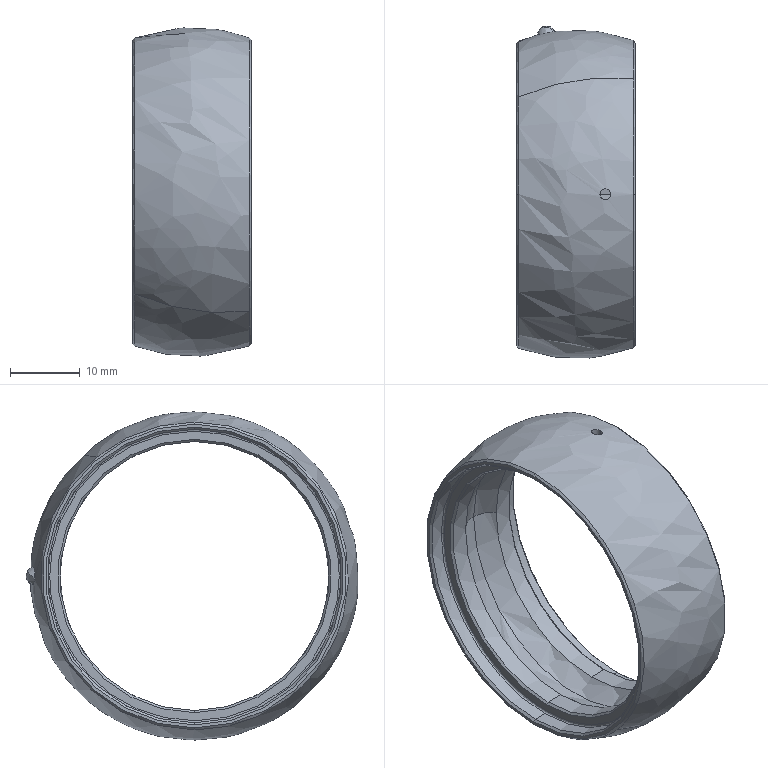Part | STEP file | Microwave Drying Flat Conveyor-inafag_ucfl204_62o9y6gnj3059x015y4y3bh4_02 | 1 solid | 38 faces | box 17 x 47.603 x 47 mm | volume 6473 mm3 | spline 12 | cone 12 | cylinder 10 | plane 4 | commonest cylinder face diameters 38.5 x4 42 x4 1.545 x2